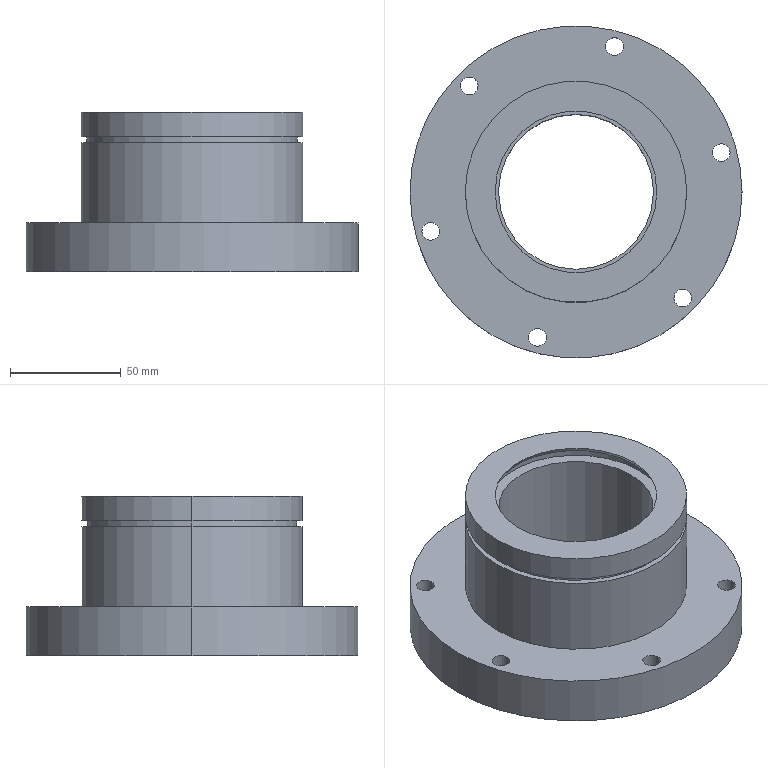Part | SolidWorks | features ICE 3, Chamfer 1, Extrusion 1, RevCut 1 | 1 solid | 45 faces | box 150 x 150 x 72 mm | volume 489629 mm3 | cylinder 24 | cone 14 | plane 7 | commonest cylinder face diameters 8 x12 100 x4 70 x2 80 x2 95 x2 150 x2
STEP:
#1=CARTESIAN_POINT('',(-40.,0.,65.7));
#2=VERTEX_POINT('',#1);
#3=CARTESIAN_POINT('',(40.,0.,65.7));
#4=VERTEX_POINT('',#3);
#5=CARTESIAN_POINT('',(0.,0.,65.7));
#6=DIRECTION('',(0.,0.,1.));
#7=DIRECTION('',(1.,0.,0.));
#8=AXIS2_PLACEMENT_3D('',#5,#6,#7);
#9=CIRCLE('',#8,40.);
#10=EDGE_CURVE('',#2,#4,#9,.T.);
#11=ORIENTED_EDGE('',*,*,#10,.F.);
#12=CARTESIAN_POINT('',(-40.,0.,70.));
#13=VERTEX_POINT('',#12);
#14=CARTESIAN_POINT('',(-40.,0.,72.));
#15=DIRECTION('',(0.,0.,1.));
#16=VECTOR('',#15,1000.);
#17=LINE('',#14,#16);
#18=EDGE_CURVE('',#2,#13,#17,.T.);
#19=ORIENTED_EDGE('',*,*,#18,.T.);
#20=CARTESIAN_POINT('',(40.,0.,70.));
#21=VERTEX_POINT('',#20);
#22=CARTESIAN_POINT('',(0.,0.,70.));
#23=DIRECTION('',(0.,0.,1.));
#24=DIRECTION('',(1.,0.,0.));
#25=AXIS2_PLACEMENT_3D('',#22,#23,#24);
#26=CIRCLE('',#25,40.);
#27=EDGE_CURVE('',#13,#21,#26,.T.);
#28=ORIENTED_EDGE('',*,*,#27,.T.);
#29=CARTESIAN_POINT('',(40.,0.,72.));
#30=DIRECTION('',(0.,0.,1.));
#31=VECTOR('',#30,1000.);
#32=LINE('',#29,#31);
#33=EDGE_CURVE('',#4,#21,#32,.T.);
#34=ORIENTED_EDGE('',*,*,#33,.F.);
#35=EDGE_LOOP('',(#11,#19,#28,#34));
#36=FACE_OUTER_BOUND('',#35,.T.);
#37=CARTESIAN_POINT('',(0.,0.,72.));
#38=DIRECTION('',(0.,0.,1.));
#39=DIRECTION('',(1.,0.,0.));
#40=AXIS2_PLACEMENT_3D('',#37,#38,#39);
#41=CYLINDRICAL_SURFACE('',#40,40.);
#42=ADVANCED_FACE('',(#36),#41,.F.);
#43=CARTESIAN_POINT('',(-36.5,0.,72.));
#44=VERTEX_POINT('',#43);
#45=CARTESIAN_POINT('',(36.5,0.,72.));
#46=VERTEX_POINT('',#45);
#47=CARTESIAN_POINT('',(0.,0.,72.));
#48=DIRECTION('',(0.,0.,1.));
#49=DIRECTION('',(1.,0.,0.));
#50=AXIS2_PLACEMENT_3D('',#47,#48,#49);
#51=CIRCLE('',#50,36.5);
#52=EDGE_CURVE('',#44,#46,#51,.T.);
#53=ORIENTED_EDGE('',*,*,#52,.T.);
#54=CARTESIAN_POINT('',(37.655,0.,70.));
#55=VERTEX_POINT('',#54);
#56=CARTESIAN_POINT('',(37.655,0.,70.));
#57=DIRECTION('',(0.5,0.,-0.866));
#58=VECTOR('',#57,1000.);
#59=LINE('',#56,#58);
#60=EDGE_CURVE('',#46,#55,#59,.T.);
#61=ORIENTED_EDGE('',*,*,#60,.T.);
#62=CARTESIAN_POINT('',(-37.655,0.,70.));
#63=VERTEX_POINT('',#62);
#64=CARTESIAN_POINT('',(0.,0.,70.));
#65=DIRECTION('',(0.,0.,1.));
#66=DIRECTION('',(1.,0.,0.));
#67=AXIS2_PLACEMENT_3D('',#64,#65,#66);
#68=CIRCLE('',#67,37.655);
#69=EDGE_CURVE('',#63,#55,#68,.T.);
#70=ORIENTED_EDGE('',*,*,#69,.F.);
#71=CARTESIAN_POINT('',(-37.655,0.,70.));
#72=DIRECTION('',(-0.5,0.,-0.866));
#73=VECTOR('',#72,1000.);
#74=LINE('',#71,#73);
#75=EDGE_CURVE('',#44,#63,#74,.T.);
#76=ORIENTED_EDGE('',*,*,#75,.F.);
#77=EDGE_LOOP('',(#53,#61,#70,#76));
#78=FACE_OUTER_BOUND('',#77,.T.);
#79=CARTESIAN_POINT('',(0.,0.,70.));
#80=DIRECTION('',(0.,0.,-1.));
#81=DIRECTION('',(-1.,0.,0.));
#82=AXIS2_PLACEMENT_3D('',#79,#80,#81);
#83=CONICAL_SURFACE('',#82,37.655,0.5236);
#84=ADVANCED_FACE('',(#78),#83,.F.);
#85=CARTESIAN_POINT('',(21.414,65.732,1.));
#86=VERTEX_POINT('',#85);
#87=CARTESIAN_POINT('',(13.414,65.732,1.));
#88=VERTEX_POINT('',#87);
#89=CARTESIAN_POINT('',(17.414,65.732,1.));
#90=DIRECTION('',(0.,0.,-1.));
#91=DIRECTION('',(1.,0.,0.));
#92=AXIS2_PLACEMENT_3D('',#89,#90,#91);
#93=CIRCLE('',#92,4.);
#94=EDGE_CURVE('',#86,#88,#93,.T.);
#95=ORIENTED_EDGE('',*,*,#94,.F.);
#96=CARTESIAN_POINT('',(22.414,65.732,0.));
#97=VERTEX_POINT('',#96);
#98=CARTESIAN_POINT('',(21.414,65.732,1.));
#99=DIRECTION('',(0.7071,0.,-0.7071));
#100=VECTOR('',#99,1000.);
#101=LINE('',#98,#100);
#102=EDGE_CURVE('',#86,#97,#101,.T.);
#103=ORIENTED_EDGE('',*,*,#102,.T.);
#104=CARTESIAN_POINT('',(12.414,65.732,0.));
#105=VERTEX_POINT('',#104);
#106=CARTESIAN_POINT('',(17.414,65.732,0.));
#107=DIRECTION('',(0.,0.,1.));
#108=DIRECTION('',(1.,0.,0.));
#109=AXIS2_PLACEMENT_3D('',#106,#107,#108);
#110=CIRCLE('',#109,5.);
#111=EDGE_CURVE('',#105,#97,#110,.T.);
#112=ORIENTED_EDGE('',*,*,#111,.F.);
#113=CARTESIAN_POINT('',(13.414,65.732,1.));
#114=DIRECTION('',(-0.7071,0.,-0.7071));
#115=VECTOR('',#114,1000.);
#116=LINE('',#113,#115);
#117=EDGE_CURVE('',#88,#105,#116,.T.);
#118=ORIENTED_EDGE('',*,*,#117,.F.);
#119=EDGE_LOOP('',(#95,#103,#112,#118));
#120=FACE_OUTER_BOUND('',#119,.T.);
#121=CARTESIAN_POINT('',(17.414,65.732,1.));
#122=DIRECTION('',(0.,0.,-1.));
#123=DIRECTION('',(-1.,0.,0.));
#124=AXIS2_PLACEMENT_3D('',#121,#122,#123);
#125=CONICAL_SURFACE('',#124,4.,0.7854);
#126=ADVANCED_FACE('',(#120),#125,.F.);
#127=CARTESIAN_POINT('',(69.633,17.785,1.));
#128=VERTEX_POINT('',#127);
#129=CARTESIAN_POINT('',(61.633,17.785,1.));
#130=VERTEX_POINT('',#129);
#131=CARTESIAN_POINT('',(65.633,17.785,1.));
#132=DIRECTION('',(0.,0.,-1.));
#133=DIRECTION('',(1.,0.,0.));
#134=AXIS2_PLACEMENT_3D('',#131,#132,#133);
#135=CIRCLE('',#134,4.);
#136=EDGE_CURVE('',#128,#130,#135,.T.);
#137=ORIENTED_EDGE('',*,*,#136,.F.);
#138=CARTESIAN_POINT('',(70.633,17.785,0.));
#139=VERTEX_POINT('',#138);
#140=CARTESIAN_POINT('',(69.633,17.785,1.));
#141=DIRECTION('',(0.7071,0.,-0.7071));
#142=VECTOR('',#141,1000.);
#143=LINE('',#140,#142);
#144=EDGE_CURVE('',#128,#139,#143,.T.);
#145=ORIENTED_EDGE('',*,*,#144,.T.);
#146=CARTESIAN_POINT('',(60.633,17.785,0.));
#147=VERTEX_POINT('',#146);
#148=CARTESIAN_POINT('',(65.633,17.785,0.));
#149=DIRECTION('',(0.,0.,1.));
#150=DIRECTION('',(1.,0.,0.));
#151=AXIS2_PLACEMENT_3D('',#148,#149,#150);
#152=CIRCLE('',#151,5.);
#153=EDGE_CURVE('',#147,#139,#152,.T.);
#154=ORIENTED_EDGE('',*,*,#153,.F.);
#155=CARTESIAN_POINT('',(61.633,17.785,1.));
#156=DIRECTION('',(-0.7071,0.,-0.7071));
#157=VECTOR('',#156,1000.);
#158=LINE('',#155,#157);
#159=EDGE_CURVE('',#130,#147,#158,.T.);
#160=ORIENTED_EDGE('',*,*,#159,.F.);
#161=EDGE_LOOP('',(#137,#145,#154,#160));
#162=FACE_OUTER_BOUND('',#161,.T.);
#163=CARTESIAN_POINT('',(65.633,17.785,1.));
#164=DIRECTION('',(0.,0.,-1.));
#165=DIRECTION('',(-1.,0.,0.));
#166=AXIS2_PLACEMENT_3D('',#163,#164,#165);
#167=CONICAL_SURFACE('',#166,4.,0.7854);
#168=ADVANCED_FACE('',(#162),#167,.F.);
#169=CARTESIAN_POINT('',(-44.219,47.947,1.));
#170=VERTEX_POINT('',#169);
#171=CARTESIAN_POINT('',(-52.219,47.947,1.));
#172=VERTEX_POINT('',#171);
#173=CARTESIAN_POINT('',(-48.219,47.947,1.));
#174=DIRECTION('',(0.,0.,-1.));
#175=DIRECTION('',(1.,0.,0.));
#176=AXIS2_PLACEMENT_3D('',#173,#174,#175);
#177=CIRCLE('',#176,4.);
#178=EDGE_CURVE('',#170,#172,#177,.T.);
#179=ORIENTED_EDGE('',*,*,#178,.F.);
#180=CARTESIAN_POINT('',(-43.219,47.947,0.));
#181=VERTEX_POINT('',#180);
#182=CARTESIAN_POINT('',(-44.219,47.947,1.));
#183=DIRECTION('',(0.7071,0.,-0.7071));
#184=VECTOR('',#183,1000.);
#185=LINE('',#182,#184);
#186=EDGE_CURVE('',#170,#181,#185,.T.);
#187=ORIENTED_EDGE('',*,*,#186,.T.);
#188=CARTESIAN_POINT('',(-53.219,47.947,0.));
#189=VERTEX_POINT('',#188);
#190=CARTESIAN_POINT('',(-48.219,47.947,0.));
#191=DIRECTION('',(0.,0.,1.));
#192=DIRECTION('',(1.,0.,0.));
#193=AXIS2_PLACEMENT_3D('',#190,#191,#192);
#194=CIRCLE('',#193,5.);
#195=EDGE_CURVE('',#189,#181,#194,.T.);
#196=ORIENTED_EDGE('',*,*,#195,.F.);
#197=CARTESIAN_POINT('',(-52.219,47.947,1.));
#198=DIRECTION('',(-0.7071,0.,-0.7071));
#199=VECTOR('',#198,1000.);
#200=LINE('',#197,#199);
#201=EDGE_CURVE('',#172,#189,#200,.T.);
#202=ORIENTED_EDGE('',*,*,#201,.F.);
#203=EDGE_LOOP('',(#179,#187,#196,#202));
#204=FACE_OUTER_BOUND('',#203,.T.);
#205=CARTESIAN_POINT('',(-48.219,47.947,1.));
#206=DIRECTION('',(0.,0.,-1.));
#207=DIRECTION('',(-1.,0.,0.));
#208=AXIS2_PLACEMENT_3D('',#205,#206,#207);
#209=CONICAL_SURFACE('',#208,4.,0.7854);
#210=ADVANCED_FACE('',(#204),#209,.F.);
#211=CARTESIAN_POINT('',(-61.633,-17.785,1.));
#212=VERTEX_POINT('',#211);
#213=CARTESIAN_POINT('',(-69.633,-17.785,1.));
#214=VERTEX_POINT('',#213);
#215=CARTESIAN_POINT('',(-65.633,-17.785,1.));
#216=DIRECTION('',(0.,0.,-1.));
#217=DIRECTION('',(1.,0.,0.));
#218=AXIS2_PLACEMENT_3D('',#215,#216,#217);
#219=CIRCLE('',#218,4.);
#220=EDGE_CURVE('',#212,#214,#219,.T.);
#221=ORIENTED_EDGE('',*,*,#220,.F.);
#222=CARTESIAN_POINT('',(-60.633,-17.785,0.));
#223=VERTEX_POINT('',#222);
#224=CARTESIAN_POINT('',(-61.633,-17.785,1.));
#225=DIRECTION('',(0.7071,0.,-0.7071));
#226=VECTOR('',#225,1000.);
#227=LINE('',#224,#226);
#228=EDGE_CURVE('',#212,#223,#227,.T.);
#229=ORIENTED_EDGE('',*,*,#228,.T.);
#230=CARTESIAN_POINT('',(-70.633,-17.785,0.));
#231=VERTEX_POINT('',#230);
#232=CARTESIAN_POINT('',(-65.633,-17.785,0.));
#233=DIRECTION('',(0.,0.,1.));
#234=DIRECTION('',(1.,0.,0.));
#235=AXIS2_PLACEMENT_3D('',#232,#233,#234);
#236=CIRCLE('',#235,5.);
#237=EDGE_CURVE('',#231,#223,#236,.T.);
#238=ORIENTED_EDGE('',*,*,#237,.F.);
#239=CARTESIAN_POINT('',(-69.633,-17.785,1.));
#240=DIRECTION('',(-0.7071,0.,-0.7071));
#241=VECTOR('',#240,1000.);
#242=LINE('',#239,#241);
#243=EDGE_CURVE('',#214,#231,#242,.T.);
#244=ORIENTED_EDGE('',*,*,#243,.F.);
#245=EDGE_LOOP('',(#221,#229,#238,#244));
#246=FACE_OUTER_BOUND('',#245,.T.);
#247=CARTESIAN_POINT('',(-65.633,-17.785,1.));
#248=DIRECTION('',(0.,0.,-1.));
#249=DIRECTION('',(-1.,0.,0.));
#250=AXIS2_PLACEMENT_3D('',#247,#248,#249);
#251=CONICAL_SURFACE('',#250,4.,0.7854);
#252=ADVANCED_FACE('',(#246),#251,.F.);
#253=CARTESIAN_POINT('',(-13.414,-65.732,1.));
#254=VERTEX_POINT('',#253);
#255=CARTESIAN_POINT('',(-21.414,-65.732,1.));
#256=VERTEX_POINT('',#255);
#257=CARTESIAN_POINT('',(-17.414,-65.732,1.));
#258=DIRECTION('',(0.,0.,-1.));
#259=DIRECTION('',(1.,0.,0.));
#260=AXIS2_PLACEMENT_3D('',#257,#258,#259);
#261=CIRCLE('',#260,4.);
#262=EDGE_CURVE('',#254,#256,#261,.T.);
#263=ORIENTED_EDGE('',*,*,#262,.F.);
#264=CARTESIAN_POINT('',(-12.414,-65.732,0.));
#265=VERTEX_POINT('',#264);
#266=CARTESIAN_POINT('',(-13.414,-65.732,1.));
#267=DIRECTION('',(0.7071,0.,-0.7071));
#268=VECTOR('',#267,1000.);
#269=LINE('',#266,#268);
#270=EDGE_CURVE('',#254,#265,#269,.T.);
#271=ORIENTED_EDGE('',*,*,#270,.T.);
#272=CARTESIAN_POINT('',(-22.414,-65.732,0.));
#273=VERTEX_POINT('',#272);
#274=CARTESIAN_POINT('',(-17.414,-65.732,0.));
#275=DIRECTION('',(0.,0.,1.));
#276=DIRECTION('',(1.,0.,0.));
#277=AXIS2_PLACEMENT_3D('',#274,#275,#276);
#278=CIRCLE('',#277,5.);
#279=EDGE_CURVE('',#273,#265,#278,.T.);
#280=ORIENTED_EDGE('',*,*,#279,.F.);
#281=CARTESIAN_POINT('',(-21.414,-65.732,1.));
#282=DIRECTION('',(-0.7071,0.,-0.7071));
#283=VECTOR('',#282,1000.);
#284=LINE('',#281,#283);
#285=EDGE_CURVE('',#256,#273,#284,.T.);
#286=ORIENTED_EDGE('',*,*,#285,.F.);
#287=EDGE_LOOP('',(#263,#271,#280,#286));
#288=FACE_OUTER_BOUND('',#287,.T.);
#289=CARTESIAN_POINT('',(-17.414,-65.732,1.));
#290=DIRECTION('',(0.,0.,-1.));
#291=DIRECTION('',(-1.,0.,0.));
#292=AXIS2_PLACEMENT_3D('',#289,#290,#291);
#293=CONICAL_SURFACE('',#292,4.,0.7854);
#294=ADVANCED_FACE('',(#288),#293,.F.);
#295=CARTESIAN_POINT('',(52.219,-47.947,1.));
#296=VERTEX_POINT('',#295);
#297=CARTESIAN_POINT('',(44.219,-47.947,1.));
#298=VERTEX_POINT('',#297);
#299=CARTESIAN_POINT('',(48.219,-47.947,1.));
#300=DIRECTION('',(0.,0.,-1.));
#301=DIRECTION('',(1.,0.,0.));
#302=AXIS2_PLACEMENT_3D('',#299,#300,#301);
#303=CIRCLE('',#302,4.);
#304=EDGE_CURVE('',#296,#298,#303,.T.);
#305=ORIENTED_EDGE('',*,*,#304,.F.);
#306=CARTESIAN_POINT('',(53.219,-47.947,0.));
#307=VERTEX_POINT('',#306);
#308=CARTESIAN_POINT('',(52.219,-47.947,1.));
#309=DIRECTION('',(0.7071,0.,-0.7071));
#310=VECTOR('',#309,1000.);
#311=LINE('',#308,#310);
#312=EDGE_CURVE('',#296,#307,#311,.T.);
#313=ORIENTED_EDGE('',*,*,#312,.T.);
#314=CARTESIAN_POINT('',(43.219,-47.947,0.));
#315=VERTEX_POINT('',#314);
#316=CARTESIAN_POINT('',(48.219,-47.947,0.));
#317=DIRECTION('',(0.,0.,1.));
#318=DIRECTION('',(1.,0.,0.));
#319=AXIS2_PLACEMENT_3D('',#316,#317,#318);
#320=CIRCLE('',#319,5.);
#321=EDGE_CURVE('',#315,#307,#320,.T.);
#322=ORIENTED_EDGE('',*,*,#321,.F.);
#323=CARTESIAN_POINT('',(44.219,-47.947,1.));
#324=DIRECTION('',(-0.7071,0.,-0.7071));
#325=VECTOR('',#324,1000.);
#326=LINE('',#323,#325);
#327=EDGE_CURVE('',#298,#315,#326,.T.);
#328=ORIENTED_EDGE('',*,*,#327,.F.);
#329=EDGE_LOOP('',(#305,#313,#322,#328));
#330=FACE_OUTER_BOUND('',#329,.T.);
#331=CARTESIAN_POINT('',(48.219,-47.947,1.));
#332=DIRECTION('',(0.,0.,-1.));
#333=DIRECTION('',(-1.,0.,0.));
#334=AXIS2_PLACEMENT_3D('',#331,#332,#333);
#335=CONICAL_SURFACE('',#334,4.,0.7854);
#336=ADVANCED_FACE('',(#330),#335,.F.);
#337=CARTESIAN_POINT('',(13.414,65.732,22.));
#338=VERTEX_POINT('',#337);
#339=CARTESIAN_POINT('',(21.414,65.732,22.));
#340=VERTEX_POINT('',#339);
#341=CARTESIAN_POINT('',(17.414,65.732,22.));
#342=DIRECTION('',(0.,0.,1.));
#343=DIRECTION('',(1.,0.,0.));
#344=AXIS2_PLACEMENT_3D('',#341,#342,#343);
#345=CIRCLE('',#344,4.);
#346=EDGE_CURVE('',#338,#340,#345,.T.);
#347=ORIENTED_EDGE('',*,*,#346,.T.);
#348=CARTESIAN_POINT('',(21.414,65.732,72.));
#349=DIRECTION('',(0.,0.,-1.));
#350=VECTOR('',#349,1000.);
#351=LINE('',#348,#350);
#352=EDGE_CURVE('',#340,#86,#351,.T.);
#353=ORIENTED_EDGE('',*,*,#352,.T.);
#354=ORIENTED_EDGE('',*,*,#94,.T.);
#355=CARTESIAN_POINT('',(13.414,65.732,72.));
#356=DIRECTION('',(0.,0.,-1.));
#357=VECTOR('',#356,1000.);
#358=LINE('',#355,#357);
#359=EDGE_CURVE('',#338,#88,#358,.T.);
#360=ORIENTED_EDGE('',*,*,#359,.F.);
#361=EDGE_LOOP('',(#347,#353,#354,#360));
#362=FACE_OUTER_BOUND('',#361,.T.);
#363=CARTESIAN_POINT('',(17.414,65.732,72.));
#364=DIRECTION('',(0.,0.,-1.));
#365=DIRECTION('',(-1.,0.,0.));
#366=AXIS2_PLACEMENT_3D('',#363,#364,#365);
#367=CYLINDRICAL_SURFACE('',#366,4.);
#368=ADVANCED_FACE('',(#362),#367,.F.);
#369=CARTESIAN_POINT('',(-52.219,47.947,22.));
#370=VERTEX_POINT('',#369);
#371=CARTESIAN_POINT('',(-44.219,47.947,22.));
#372=VERTEX_POINT('',#371);
#373=CARTESIAN_POINT('',(-48.219,47.947,22.));
#374=DIRECTION('',(0.,0.,1.));
#375=DIRECTION('',(1.,0.,0.));
#376=AXIS2_PLACEMENT_3D('',#373,#374,#375);
#377=CIRCLE('',#376,4.);
#378=EDGE_CURVE('',#370,#372,#377,.T.);
#379=ORIENTED_EDGE('',*,*,#378,.T.);
#380=CARTESIAN_POINT('',(-44.219,47.947,72.));
#381=DIRECTION('',(0.,0.,-1.));
#382=VECTOR('',#381,1000.);
#383=LINE('',#380,#382);
#384=EDGE_CURVE('',#372,#170,#383,.T.);
#385=ORIENTED_EDGE('',*,*,#384,.T.);
#386=ORIENTED_EDGE('',*,*,#178,.T.);
#387=CARTESIAN_POINT('',(-52.219,47.947,72.));
#388=DIRECTION('',(0.,0.,-1.));
#389=VECTOR('',#388,1000.);
#390=LINE('',#387,#389);
#391=EDGE_CURVE('',#370,#172,#390,.T.);
#392=ORIENTED_EDGE('',*,*,#391,.F.);
#393=EDGE_LOOP('',(#379,#385,#386,#392));
#394=FACE_OUTER_BOUND('',#393,.T.);
#395=CARTESIAN_POINT('',(-48.219,47.947,72.));
#396=DIRECTION('',(0.,0.,-1.));
#397=DIRECTION('',(-1.,0.,0.));
#398=AXIS2_PLACEMENT_3D('',#395,#396,#397);
#399=CYLINDRICAL_SURFACE('',#398,4.);
#400=ADVANCED_FACE('',(#394),#399,.F.);
#401=CARTESIAN_POINT('',(-69.633,-17.785,22.));
#402=VERTEX_POINT('',#401);
#403=CARTESIAN_POINT('',(-61.633,-17.785,22.));
#404=VERTEX_POINT('',#403);
#405=CARTESIAN_POINT('',(-65.633,-17.785,22.));
#406=DIRECTION('',(0.,0.,1.));
#407=DIRECTION('',(1.,0.,0.));
#408=AXIS2_PLACEMENT_3D('',#405,#406,#407);
#409=CIRCLE('',#408,4.);
#410=EDGE_CURVE('',#402,#404,#409,.T.);
#411=ORIENTED_EDGE('',*,*,#410,.T.);
#412=CARTESIAN_POINT('',(-61.633,-17.785,72.));
#413=DIRECTION('',(0.,0.,-1.));
#414=VECTOR('',#413,1000.);
#415=LINE('',#412,#414);
#416=EDGE_CURVE('',#404,#212,#415,.T.);
#417=ORIENTED_EDGE('',*,*,#416,.T.);
#418=ORIENTED_EDGE('',*,*,#220,.T.);
#419=CARTESIAN_POINT('',(-69.633,-17.785,72.));
#420=DIRECTION('',(0.,0.,-1.));
#421=VECTOR('',#420,1000.);
#422=LINE('',#419,#421);
#423=EDGE_CURVE('',#402,#214,#422,.T.);
#424=ORIENTED_EDGE('',*,*,#423,.F.);
#425=EDGE_LOOP('',(#411,#417,#418,#424));
#426=FACE_OUTER_BOUND('',#425,.T.);
#427=CARTESIAN_POINT('',(-65.633,-17.785,72.));
#428=DIRECTION('',(0.,0.,-1.));
#429=DIRECTION('',(-1.,0.,0.));
#430=AXIS2_PLACEMENT_3D('',#427,#428,#429);
#431=CYLINDRICAL_SURFACE('',#430,4.);
#432=ADVANCED_FACE('',(#426),#431,.F.);
#433=CARTESIAN_POINT('',(-21.414,-65.732,22.));
#434=VERTEX_POINT('',#433);
#435=CARTESIAN_POINT('',(-13.414,-65.732,22.));
#436=VERTEX_POINT('',#435);
#437=CARTESIAN_POINT('',(-17.414,-65.732,22.));
#438=DIRECTION('',(0.,0.,1.));
#439=DIRECTION('',(1.,0.,0.));
#440=AXIS2_PLACEMENT_3D('',#437,#438,#439);
#441=CIRCLE('',#440,4.);
#442=EDGE_CURVE('',#434,#436,#441,.T.);
#443=ORIENTED_EDGE('',*,*,#442,.T.);
#444=CARTESIAN_POINT('',(-13.414,-65.732,72.));
#445=DIRECTION('',(0.,0.,-1.));
#446=VECTOR('',#445,1000.);
#447=LINE('',#444,#446);
#448=EDGE_CURVE('',#436,#254,#447,.T.);
#449=ORIENTED_EDGE('',*,*,#448,.T.);
#450=ORIENTED_EDGE('',*,*,#262,.T.);
#451=CARTESIAN_POINT('',(-21.414,-65.732,72.));
#452=DIRECTION('',(0.,0.,-1.));
#453=VECTOR('',#452,1000.);
#454=LINE('',#451,#453);
#455=EDGE_CURVE('',#434,#256,#454,.T.);
#456=ORIENTED_EDGE('',*,*,#455,.F.);
#457=EDGE_LOOP('',(#443,#449,#450,#456));
#458=FACE_OUTER_BOUND('',#457,.T.);
#459=CARTESIAN_POINT('',(-17.414,-65.732,72.));
#460=DIRECTION('',(0.,0.,-1.));
#461=DIRECTION('',(-1.,0.,0.));
#462=AXIS2_PLACEMENT_3D('',#459,#460,#461);
#463=CYLINDRICAL_SURFACE('',#462,4.);
#464=ADVANCED_FACE('',(#458),#463,.F.);
#465=CARTESIAN_POINT('',(44.219,-47.947,22.));
#466=VERTEX_POINT('',#465);
#467=CARTESIAN_POINT('',(52.219,-47.947,22.));
#468=VERTEX_POINT('',#467);
#469=CARTESIAN_POINT('',(48.219,-47.947,22.));
#470=DIRECTION('',(0.,0.,1.));
#471=DIRECTION('',(1.,0.,0.));
#472=AXIS2_PLACEMENT_3D('',#469,#470,#471);
#473=CIRCLE('',#472,4.);
#474=EDGE_CURVE('',#466,#468,#473,.T.);
#475=ORIENTED_EDGE('',*,*,#474,.T.);
#476=CARTESIAN_POINT('',(52.219,-47.947,72.));
#477=DIRECTION('',(0.,0.,-1.));
#478=VECTOR('',#477,1000.);
#479=LINE('',#476,#478);
#480=EDGE_CURVE('',#468,#296,#479,.T.);
#481=ORIENTED_EDGE('',*,*,#480,.T.);
#482=ORIENTED_EDGE('',*,*,#304,.T.);
#483=CARTESIAN_POINT('',(44.219,-47.947,72.));
#484=DIRECTION('',(0.,0.,-1.));
#485=VECTOR('',#484,1000.);
#486=LINE('',#483,#485);
#487=EDGE_CURVE('',#466,#298,#486,.T.);
#488=ORIENTED_EDGE('',*,*,#487,.F.);
#489=EDGE_LOOP('',(#475,#481,#482,#488));
#490=FACE_OUTER_BOUND('',#489,.T.);
#491=CARTESIAN_POINT('',(48.219,-47.947,72.));
#492=DIRECTION('',(0.,0.,-1.));
#493=DIRECTION('',(-1.,0.,0.));
#494=AXIS2_PLACEMENT_3D('',#491,#492,#493);
#495=CYLINDRICAL_SURFACE('',#494,4.);
#496=ADVANCED_FACE('',(#490),#495,.F.);
#497=CARTESIAN_POINT('',(61.633,17.785,22.));
#498=VERTEX_POINT('',#497);
#499=CARTESIAN_POINT('',(69.633,17.785,22.));
#500=VERTEX_POINT('',#499);
#501=CARTESIAN_POINT('',(65.633,17.785,22.));
#502=DIRECTION('',(0.,0.,1.));
#503=DIRECTION('',(1.,0.,0.));
#504=AXIS2_PLACEMENT_3D('',#501,#502,#503);
#505=CIRCLE('',#504,4.);
#506=EDGE_CURVE('',#498,#500,#505,.T.);
#507=ORIENTED_EDGE('',*,*,#506,.T.);
#508=CARTESIAN_POINT('',(69.633,17.785,72.));
#509=DIRECTION('',(0.,0.,-1.));
#510=VECTOR('',#509,1000.);
#511=LINE('',#508,#510);
#512=EDGE_CURVE('',#500,#128,#511,.T.);
#513=ORIENTED_EDGE('',*,*,#512,.T.);
#514=ORIENTED_EDGE('',*,*,#136,.T.);
#515=CARTESIAN_POINT('',(61.633,17.785,72.));
#516=DIRECTION('',(0.,0.,-1.));
#517=VECTOR('',#516,1000.);
#518=LINE('',#515,#517);
#519=EDGE_CURVE('',#498,#130,#518,.T.);
#520=ORIENTED_EDGE('',*,*,#519,.F.);
#521=EDGE_LOOP('',(#507,#513,#514,#520));
#522=FACE_OUTER_BOUND('',#521,.T.);
#523=CARTESIAN_POINT('',(65.633,17.785,72.));
#524=DIRECTION('',(0.,0.,-1.));
#525=DIRECTION('',(-1.,0.,0.));
#526=AXIS2_PLACEMENT_3D('',#523,#524,#525);
#527=CYLINDRICAL_SURFACE('',#526,4.);
#528=ADVANCED_FACE('',(#522),#527,.F.);
#529=CARTESIAN_POINT('',(47.5,0.,58.35));
#530=VERTEX_POINT('',#529);
#531=CARTESIAN_POINT('',(-47.5,0.,58.35));
#532=VERTEX_POINT('',#531);
#533=CARTESIAN_POINT('',(0.,0.,58.35));
#534=DIRECTION('',(0.,0.,1.));
#535=DIRECTION('',(1.,0.,0.));
#536=AXIS2_PLACEMENT_3D('',#533,#534,#535);
#537=CIRCLE('',#536,47.5);
#538=EDGE_CURVE('',#530,#532,#537,.T.);
#539=ORIENTED_EDGE('',*,*,#538,.T.);
#540=CARTESIAN_POINT('',(-47.5,0.,61.));
#541=VERTEX_POINT('',#540);
#542=CARTESIAN_POINT('',(-47.5,0.,58.35));
#543=DIRECTION('',(0.,0.,1.));
#544=VECTOR('',#543,1000.);
#545=LINE('',#542,#544);
#546=EDGE_CURVE('',#532,#541,#545,.T.);
#547=ORIENTED_EDGE('',*,*,#546,.T.);
#548=CARTESIAN_POINT('',(47.5,0.,61.));
#549=VERTEX_POINT('',#548);
#550=CARTESIAN_POINT('',(0.,0.,61.));
#551=DIRECTION('',(0.,0.,1.));
#552=DIRECTION('',(1.,0.,0.));
#553=AXIS2_PLACEMENT_3D('',#550,#551,#552);
#554=CIRCLE('',#553,47.5);
#555=EDGE_CURVE('',#549,#541,#554,.T.);
#556=ORIENTED_EDGE('',*,*,#555,.F.);
#557=CARTESIAN_POINT('',(47.5,0.,58.35));
#558=DIRECTION('',(0.,0.,1.));
#559=VECTOR('',#558,1000.);
#560=LINE('',#557,#559);
#561=EDGE_CURVE('',#530,#549,#560,.T.);
#562=ORIENTED_EDGE('',*,*,#561,.F.);
#563=EDGE_LOOP('',(#539,#547,#556,#562));
#564=FACE_OUTER_BOUND('',#563,.T.);
#565=CARTESIAN_POINT('',(0.,0.,58.35));
#566=DIRECTION('',(0.,0.,1.));
#567=DIRECTION('',(1.,0.,0.));
#568=AXIS2_PLACEMENT_3D('',#565,#566,#567);
#569=CYLINDRICAL_SURFACE('',#568,47.5);
#570=ADVANCED_FACE('',(#564),#569,.T.);
#571=CARTESIAN_POINT('',(50.,0.,72.));
#572=VERTEX_POINT('',#571);
#573=CARTESIAN_POINT('',(-50.,0.,72.));
#574=VERTEX_POINT('',#573);
#575=CARTESIAN_POINT('',(0.,0.,72.));
#576=DIRECTION('',(0.,0.,1.));
#577=DIRECTION('',(1.,0.,0.));
#578=AXIS2_PLACEMENT_3D('',#575,#576,#577);
#579=CIRCLE('',#578,50.);
#580=EDGE_CURVE('',#572,#574,#579,.T.);
#581=ORIENTED_EDGE('',*,*,#580,.F.);
#582=CARTESIAN_POINT('',(50.,0.,61.));
#583=VERTEX_POINT('',#582);
#584=CARTESIAN_POINT('',(50.,0.,72.));
#585=DIRECTION('',(0.,0.,-1.));
#586=VECTOR('',#585,1000.);
#587=LINE('',#584,#586);
#588=EDGE_CURVE('',#572,#583,#587,.T.);
#589=ORIENTED_EDGE('',*,*,#588,.T.);
#590=CARTESIAN_POINT('',(-50.,0.,61.));
#591=VERTEX_POINT('',#590);
#592=CARTESIAN_POINT('',(0.,0.,61.));
#593=DIRECTION('',(0.,0.,1.));
#594=DIRECTION('',(1.,0.,0.));
#595=AXIS2_PLACEMENT_3D('',#592,#593,#594);
#596=CIRCLE('',#595,50.);
#597=EDGE_CURVE('',#583,#591,#596,.T.);
#598=ORIENTED_EDGE('',*,*,#597,.T.);
#599=CARTESIAN_POINT('',(-50.,0.,72.));
#600=DIRECTION('',(0.,0.,-1.));
#601=VECTOR('',#600,1000.);
#602=LINE('',#599,#601);
#603=EDGE_CURVE('',#574,#591,#602,.T.);
#604=ORIENTED_EDGE('',*,*,#603,.F.);
#605=EDGE_LOOP('',(#581,#589,#598,#604));
#606=FACE_OUTER_BOUND('',#605,.T.);
#607=CARTESIAN_POINT('',(0.,0.,72.));
#608=DIRECTION('',(0.,0.,-1.));
#609=DIRECTION('',(-1.,0.,0.));
#610=AXIS2_PLACEMENT_3D('',#607,#608,#609);
#611=CYLINDRICAL_SURFACE('',#610,50.);
#612=ADVANCED_FACE('',(#606),#611,.T.);
#613=CARTESIAN_POINT('',(75.,0.,22.));
#614=VERTEX_POINT('',#613);
#615=CARTESIAN_POINT('',(-75.,0.,22.));
#616=VERTEX_POINT('',#615);
#617=CARTESIAN_POINT('',(0.,0.,22.));
#618=DIRECTION('',(0.,0.,1.));
#619=DIRECTION('',(1.,0.,0.));
#620=AXIS2_PLACEMENT_3D('',#617,#618,#619);
#621=CIRCLE('',#620,75.);
#622=EDGE_CURVE('',#614,#616,#621,.T.);
#623=ORIENTED_EDGE('',*,*,#622,.F.);
#624=CARTESIAN_POINT('',(75.,0.,0.));
#625=VERTEX_POINT('',#624);
#626=CARTESIAN_POINT('',(75.,0.,22.));
#627=DIRECTION('',(0.,0.,-1.));
#628=VECTOR('',#627,1000.);
#629=LINE('',#626,#628);
#630=EDGE_CURVE('',#614,#625,#629,.T.);
#631=ORIENTED_EDGE('',*,*,#630,.T.);
#632=CARTESIAN_POINT('',(-75.,0.,0.));
#633=VERTEX_POINT('',#632);
#634=CARTESIAN_POINT('',(0.,0.,0.));
#635=DIRECTION('',(0.,0.,1.));
#636=DIRECTION('',(1.,0.,0.));
#637=AXIS2_PLACEMENT_3D('',#634,#635,#636);
#638=CIRCLE('',#637,75.);
#639=EDGE_CURVE('',#625,#633,#638,.T.);
#640=ORIENTED_EDGE('',*,*,#639,.T.);
#641=CARTESIAN_POINT('',(-75.,0.,22.));
#642=DIRECTION('',(0.,0.,-1.));
#643=VECTOR('',#642,1000.);
#644=LINE('',#641,#643);
#645=EDGE_CURVE('',#616,#633,#644,.T.);
#646=ORIENTED_EDGE('',*,*,#645,.F.);
#647=EDGE_LOOP('',(#623,#631,#640,#646));
#648=FACE_OUTER_BOUND('',#647,.T.);
#649=CARTESIAN_POINT('',(0.,0.,22.));
#650=DIRECTION('',(0.,0.,-1.));
#651=DIRECTION('',(-1.,0.,0.));
#652=AXIS2_PLACEMENT_3D('',#649,#650,#651);
#653=CYLINDRICAL_SURFACE('',#652,75.);
#654=ADVANCED_FACE('',(#648),#653,.T.);
#655=CARTESIAN_POINT('',(50.,0.,58.35));
#656=VERTEX_POINT('',#655);
#657=CARTESIAN_POINT('',(-50.,0.,58.35));
#658=VERTEX_POINT('',#657);
#659=CARTESIAN_POINT('',(0.,0.,58.35));
#660=DIRECTION('',(0.,0.,1.));
#661=DIRECTION('',(1.,0.,0.));
#662=AXIS2_PLACEMENT_3D('',#659,#660,#661);
#663=CIRCLE('',#662,50.);
#664=EDGE_CURVE('',#656,#658,#663,.T.);
#665=ORIENTED_EDGE('',*,*,#664,.F.);
#666=CARTESIAN_POINT('',(50.,0.,22.));
#667=VERTEX_POINT('',#666);
#668=CARTESIAN_POINT('',(50.,0.,72.));
#669=DIRECTION('',(0.,0.,-1.));
#670=VECTOR('',#669,1000.);
#671=LINE('',#668,#670);
#672=EDGE_CURVE('',#656,#667,#671,.T.);
#673=ORIENTED_EDGE('',*,*,#672,.T.);
#674=CARTESIAN_POINT('',(-50.,0.,22.));
#675=VERTEX_POINT('',#674);
#676=CARTESIAN_POINT('',(0.,0.,22.));
#677=DIRECTION('',(0.,0.,1.));
#678=DIRECTION('',(1.,0.,0.));
#679=AXIS2_PLACEMENT_3D('',#676,#677,#678);
#680=CIRCLE('',#679,50.);
#681=EDGE_CURVE('',#667,#675,#680,.T.);
#682=ORIENTED_EDGE('',*,*,#681,.T.);
#683=CARTESIAN_POINT('',(-50.,0.,72.));
#684=DIRECTION('',(0.,0.,-1.));
#685=VECTOR('',#684,1000.);
#686=LINE('',#683,#685);
#687=EDGE_CURVE('',#658,#675,#686,.T.);
#688=ORIENTED_EDGE('',*,*,#687,.F.);
#689=EDGE_LOOP('',(#665,#673,#682,#688));
#690=FACE_OUTER_BOUND('',#689,.T.);
#691=CARTESIAN_POINT('',(0.,0.,72.));
#692=DIRECTION('',(0.,0.,-1.));
#693=DIRECTION('',(-1.,0.,0.));
#694=AXIS2_PLACEMENT_3D('',#691,#692,#693);
#695=CYLINDRICAL_SURFACE('',#694,50.);
#696=ADVANCED_FACE('',(#690),#695,.T.);
#697=CARTESIAN_POINT('',(-35.,0.,65.7));
#698=VERTEX_POINT('',#697);
#699=CARTESIAN_POINT('',(35.,0.,65.7));
#700=VERTEX_POINT('',#699);
#701=CARTESIAN_POINT('',(0.,0.,65.7));
#702=DIRECTION('',(0.,0.,1.));
#703=DIRECTION('',(1.,0.,0.));
#704=AXIS2_PLACEMENT_3D('',#701,#702,#703);
#705=CIRCLE('',#704,35.);
#706=EDGE_CURVE('',#698,#700,#705,.T.);
#707=ORIENTED_EDGE('',*,*,#706,.T.);
#708=CARTESIAN_POINT('',(35.,0.,0.));
#709=VERTEX_POINT('',#708);
#710=CARTESIAN_POINT('',(35.,0.,22.));
#711=DIRECTION('',(0.,0.,-1.));
#712=VECTOR('',#711,1000.);
#713=LINE('',#710,#712);
#714=EDGE_CURVE('',#700,#709,#713,.T.);
#715=ORIENTED_EDGE('',*,*,#714,.T.);
#716=CARTESIAN_POINT('',(-35.,0.,0.));
#717=VERTEX_POINT('',#716);
#718=CARTESIAN_POINT('',(0.,0.,0.));
#719=DIRECTION('',(0.,0.,1.));
#720=DIRECTION('',(1.,0.,0.));
#721=AXIS2_PLACEMENT_3D('',#718,#719,#720);
#722=CIRCLE('',#721,35.);
#723=EDGE_CURVE('',#717,#709,#722,.T.);
#724=ORIENTED_EDGE('',*,*,#723,.F.);
#725=CARTESIAN_POINT('',(-35.,0.,22.));
#726=DIRECTION('',(0.,0.,-1.));
#727=VECTOR('',#726,1000.);
#728=LINE('',#725,#727);
#729=EDGE_CURVE('',#698,#717,#728,.T.);
#730=ORIENTED_EDGE('',*,*,#729,.F.);
#731=EDGE_LOOP('',(#707,#715,#724,#730));
#732=FACE_OUTER_BOUND('',#731,.T.);
#733=CARTESIAN_POINT('',(0.,0.,22.));
#734=DIRECTION('',(0.,0.,-1.));
#735=DIRECTION('',(-1.,0.,0.));
#736=AXIS2_PLACEMENT_3D('',#733,#734,#735);
#737=CYLINDRICAL_SURFACE('',#736,35.);
#738=ADVANCED_FACE('',(#732),#737,.F.);
#739=ORIENTED_EDGE('',*,*,#714,.F.);
#740=CARTESIAN_POINT('',(0.,0.,65.7));
#741=DIRECTION('',(0.,0.,1.));
#742=DIRECTION('',(1.,0.,0.));
#743=AXIS2_PLACEMENT_3D('',#740,#741,#742);
#744=CIRCLE('',#743,35.);
#745=EDGE_CURVE('',#700,#698,#744,.T.);
#746=ORIENTED_EDGE('',*,*,#745,.T.);
#747=ORIENTED_EDGE('',*,*,#729,.T.);
#748=CARTESIAN_POINT('',(0.,0.,0.));
#749=DIRECTION('',(0.,0.,1.));
#750=DIRECTION('',(1.,0.,0.));
#751=AXIS2_PLACEMENT_3D('',#748,#749,#750);
#752=CIRCLE('',#751,35.);
#753=EDGE_CURVE('',#709,#717,#752,.T.);
#754=ORIENTED_EDGE('',*,*,#753,.F.);
#755=EDGE_LOOP('',(#739,#746,#747,#754));
#756=FACE_OUTER_BOUND('',#755,.T.);
#757=CARTESIAN_POINT('',(0.,0.,22.));
#758=DIRECTION('',(0.,0.,-1.));
#759=DIRECTION('',(-1.,0.,0.));
#760=AXIS2_PLACEMENT_3D('',#757,#758,#759);
#761=CYLINDRICAL_SURFACE('',#760,35.);
#762=ADVANCED_FACE('',(#756),#761,.F.);
#763=ORIENTED_EDGE('',*,*,#672,.F.);
#764=CARTESIAN_POINT('',(0.,0.,58.35));
#765=DIRECTION('',(0.,0.,1.));
#766=DIRECTION('',(1.,0.,0.));
#767=AXIS2_PLACEMENT_3D('',#764,#765,#766);
#768=CIRCLE('',#767,50.);
#769=EDGE_CURVE('',#658,#656,#768,.T.);
#770=ORIENTED_EDGE('',*,*,#769,.F.);
#771=ORIENTED_EDGE('',*,*,#687,.T.);
#772=CARTESIAN_POINT('',(0.,0.,22.));
#773=DIRECTION('',(0.,0.,1.));
#774=DIRECTION('',(1.,0.,0.));
#775=AXIS2_PLACEMENT_3D('',#772,#773,#774);
#776=CIRCLE('',#775,50.);
#777=EDGE_CURVE('',#675,#667,#776,.T.);
#778=ORIENTED_EDGE('',*,*,#777,.T.);
#779=EDGE_LOOP('',(#763,#770,#771,#778));
#780=FACE_OUTER_BOUND('',#779,.T.);
#781=CARTESIAN_POINT('',(0.,0.,72.));
#782=DIRECTION('',(0.,0.,-1.));
#783=DIRECTION('',(-1.,0.,0.));
#784=AXIS2_PLACEMENT_3D('',#781,#782,#783);
#785=CYLINDRICAL_SURFACE('',#784,50.);
#786=ADVANCED_FACE('',(#780),#785,.T.);
#787=ORIENTED_EDGE('',*,*,#346,.F.);
#788=CARTESIAN_POINT('',(17.414,65.732,22.));
#789=DIRECTION('',(0.,0.,1.));
#790=DIRECTION('',(1.,0.,0.));
#791=AXIS2_PLACEMENT_3D('',#788,#789,#790);
#792=CIRCLE('',#791,4.);
#793=EDGE_CURVE('',#340,#338,#792,.T.);
#794=ORIENTED_EDGE('',*,*,#793,.F.);
#795=EDGE_LOOP('',(#787,#794));
#796=FACE_BOUND('',#795,.T.);
#797=ORIENTED_EDGE('',*,*,#378,.F.);
#798=CARTESIAN_POINT('',(-48.219,47.947,22.));
#799=DIRECTION('',(0.,0.,1.));
#800=DIRECTION('',(1.,0.,0.));
#801=AXIS2_PLACEMENT_3D('',#798,#799,#800);
#802=CIRCLE('',#801,4.);
#803=EDGE_CURVE('',#372,#370,#802,.T.);
#804=ORIENTED_EDGE('',*,*,#803,.F.);
#805=EDGE_LOOP('',(#797,#804));
#806=FACE_BOUND('',#805,.T.);
#807=ORIENTED_EDGE('',*,*,#410,.F.);
#808=CARTESIAN_POINT('',(-65.633,-17.785,22.));
#809=DIRECTION('',(0.,0.,1.));
#810=DIRECTION('',(1.,0.,0.));
#811=AXIS2_PLACEMENT_3D('',#808,#809,#810);
#812=CIRCLE('',#811,4.);
#813=EDGE_CURVE('',#404,#402,#812,.T.);
#814=ORIENTED_EDGE('',*,*,#813,.F.);
#815=EDGE_LOOP('',(#807,#814));
#816=FACE_BOUND('',#815,.T.);
#817=ORIENTED_EDGE('',*,*,#442,.F.);
#818=CARTESIAN_POINT('',(-17.414,-65.732,22.));
#819=DIRECTION('',(0.,0.,1.));
#820=DIRECTION('',(1.,0.,0.));
#821=AXIS2_PLACEMENT_3D('',#818,#819,#820);
#822=CIRCLE('',#821,4.);
#823=EDGE_CURVE('',#436,#434,#822,.T.);
#824=ORIENTED_EDGE('',*,*,#823,.F.);
#825=EDGE_LOOP('',(#817,#824));
#826=FACE_BOUND('',#825,.T.);
#827=ORIENTED_EDGE('',*,*,#474,.F.);
#828=CARTESIAN_POINT('',(48.219,-47.947,22.));
#829=DIRECTION('',(0.,0.,1.));
#830=DIRECTION('',(1.,0.,0.));
#831=AXIS2_PLACEMENT_3D('',#828,#829,#830);
#832=CIRCLE('',#831,4.);
#833=EDGE_CURVE('',#468,#466,#832,.T.);
#834=ORIENTED_EDGE('',*,*,#833,.F.);
#835=EDGE_LOOP('',(#827,#834));
#836=FACE_BOUND('',#835,.T.);
#837=ORIENTED_EDGE('',*,*,#506,.F.);
#838=CARTESIAN_POINT('',(65.633,17.785,22.));
#839=DIRECTION('',(0.,0.,1.));
#840=DIRECTION('',(1.,0.,0.));
#841=AXIS2_PLACEMENT_3D('',#838,#839,#840);
#842=CIRCLE('',#841,4.);
#843=EDGE_CURVE('',#500,#498,#842,.T.);
#844=ORIENTED_EDGE('',*,*,#843,.F.);
#845=EDGE_LOOP('',(#837,#844));
#846=FACE_BOUND('',#845,.T.);
#847=CARTESIAN_POINT('',(0.,0.,22.));
#848=DIRECTION('',(0.,0.,1.));
#849=DIRECTION('',(1.,0.,0.));
#850=AXIS2_PLACEMENT_3D('',#847,#848,#849);
#851=CIRCLE('',#850,75.);
#852=EDGE_CURVE('',#616,#614,#851,.T.);
#853=ORIENTED_EDGE('',*,*,#852,.T.);
#854=ORIENTED_EDGE('',*,*,#622,.T.);
#855=EDGE_LOOP('',(#853,#854));
#856=FACE_OUTER_BOUND('',#855,.T.);
#857=ORIENTED_EDGE('',*,*,#777,.F.);
#858=ORIENTED_EDGE('',*,*,#681,.F.);
#859=EDGE_LOOP('',(#857,#858));
#860=FACE_BOUND('',#859,.T.);
#861=CARTESIAN_POINT('',(0.,0.,22.));
#862=DIRECTION('',(0.,0.,1.));
#863=DIRECTION('',(1.,0.,0.));
#864=AXIS2_PLACEMENT_3D('',#861,#862,#863);
#865=PLANE('',#864);
#866=ADVANCED_FACE('',(#796,#806,#816,#826,#836,#846,#856,#860),#865,.T.);
#867=ORIENTED_EDGE('',*,*,#321,.T.);
#868=CARTESIAN_POINT('',(48.219,-47.947,0.));
#869=DIRECTION('',(0.,0.,1.));
#870=DIRECTION('',(1.,0.,0.));
#871=AXIS2_PLACEMENT_3D('',#868,#869,#870);
#872=CIRCLE('',#871,5.);
#873=EDGE_CURVE('',#307,#315,#872,.T.);
#874=ORIENTED_EDGE('',*,*,#873,.T.);
#875=EDGE_LOOP('',(#867,#874));
#876=FACE_BOUND('',#875,.T.);
#877=ORIENTED_EDGE('',*,*,#279,.T.);
#878=CARTESIAN_POINT('',(-17.414,-65.732,0.));
#879=DIRECTION('',(0.,0.,1.));
#880=DIRECTION('',(1.,0.,0.));
#881=AXIS2_PLACEMENT_3D('',#878,#879,#880);
#882=CIRCLE('',#881,5.);
#883=EDGE_CURVE('',#265,#273,#882,.T.);
#884=ORIENTED_EDGE('',*,*,#883,.T.);
#885=EDGE_LOOP('',(#877,#884));
#886=FACE_BOUND('',#885,.T.);
#887=ORIENTED_EDGE('',*,*,#237,.T.);
#888=CARTESIAN_POINT('',(-65.633,-17.785,0.));
#889=DIRECTION('',(0.,0.,1.));
#890=DIRECTION('',(1.,0.,0.));
#891=AXIS2_PLACEMENT_3D('',#888,#889,#890);
#892=CIRCLE('',#891,5.);
#893=EDGE_CURVE('',#223,#231,#892,.T.);
#894=ORIENTED_EDGE('',*,*,#893,.T.);
#895=EDGE_LOOP('',(#887,#894));
#896=FACE_BOUND('',#895,.T.);
#897=ORIENTED_EDGE('',*,*,#195,.T.);
#898=CARTESIAN_POINT('',(-48.219,47.947,0.));
#899=DIRECTION('',(0.,0.,1.));
#900=DIRECTION('',(1.,0.,0.));
#901=AXIS2_PLACEMENT_3D('',#898,#899,#900);
#902=CIRCLE('',#901,5.);
#903=EDGE_CURVE('',#181,#189,#902,.T.);
#904=ORIENTED_EDGE('',*,*,#903,.T.);
#905=EDGE_LOOP('',(#897,#904));
#906=FACE_BOUND('',#905,.T.);
#907=ORIENTED_EDGE('',*,*,#153,.T.);
#908=CARTESIAN_POINT('',(65.633,17.785,0.));
#909=DIRECTION('',(0.,0.,1.));
#910=DIRECTION('',(1.,0.,0.));
#911=AXIS2_PLACEMENT_3D('',#908,#909,#910);
#912=CIRCLE('',#911,5.);
#913=EDGE_CURVE('',#139,#147,#912,.T.);
#914=ORIENTED_EDGE('',*,*,#913,.T.);
#915=EDGE_LOOP('',(#907,#914));
#916=FACE_BOUND('',#915,.T.);
#917=ORIENTED_EDGE('',*,*,#111,.T.);
#918=CARTESIAN_POINT('',(17.414,65.732,0.));
#919=DIRECTION('',(0.,0.,1.));
#920=DIRECTION('',(1.,0.,0.));
#921=AXIS2_PLACEMENT_3D('',#918,#919,#920);
#922=CIRCLE('',#921,5.);
#923=EDGE_CURVE('',#97,#105,#922,.T.);
#924=ORIENTED_EDGE('',*,*,#923,.T.);
#925=EDGE_LOOP('',(#917,#924));
#926=FACE_BOUND('',#925,.T.);
#927=CARTESIAN_POINT('',(0.,0.,0.));
#928=DIRECTION('',(0.,0.,1.));
#929=DIRECTION('',(1.,0.,0.));
#930=AXIS2_PLACEMENT_3D('',#927,#928,#929);
#931=CIRCLE('',#930,75.);
#932=EDGE_CURVE('',#633,#625,#931,.T.);
#933=ORIENTED_EDGE('',*,*,#932,.F.);
#934=ORIENTED_EDGE('',*,*,#639,.F.);
#935=EDGE_LOOP('',(#933,#934));
#936=FACE_OUTER_BOUND('',#935,.T.);
#937=ORIENTED_EDGE('',*,*,#723,.T.);
#938=ORIENTED_EDGE('',*,*,#753,.T.);
#939=EDGE_LOOP('',(#937,#938));
#940=FACE_BOUND('',#939,.T.);
#941=CARTESIAN_POINT('',(0.,0.,0.));
#942=DIRECTION('',(0.,0.,1.));
#943=DIRECTION('',(1.,0.,0.));
#944=AXIS2_PLACEMENT_3D('',#941,#942,#943);
#945=PLANE('',#944);
#946=ADVANCED_FACE('',(#876,#886,#896,#906,#916,#926,#936,#940),#945,.F.);
#947=ORIENTED_EDGE('',*,*,#630,.F.);
#948=ORIENTED_EDGE('',*,*,#852,.F.);
#949=ORIENTED_EDGE('',*,*,#645,.T.);
#950=ORIENTED_EDGE('',*,*,#932,.T.);
#951=EDGE_LOOP('',(#947,#948,#949,#950));
#952=FACE_OUTER_BOUND('',#951,.T.);
#953=CARTESIAN_POINT('',(0.,0.,22.));
#954=DIRECTION('',(0.,0.,-1.));
#955=DIRECTION('',(-1.,0.,0.));
#956=AXIS2_PLACEMENT_3D('',#953,#954,#955);
#957=CYLINDRICAL_SURFACE('',#956,75.);
#958=ADVANCED_FACE('',(#952),#957,.T.);
#959=ORIENTED_EDGE('',*,*,#52,.F.);
#960=CARTESIAN_POINT('',(0.,0.,72.));
#961=DIRECTION('',(0.,0.,1.));
#962=DIRECTION('',(1.,0.,0.));
#963=AXIS2_PLACEMENT_3D('',#960,#961,#962);
#964=CIRCLE('',#963,36.5);
#965=EDGE_CURVE('',#46,#44,#964,.T.);
#966=ORIENTED_EDGE('',*,*,#965,.F.);
#967=EDGE_LOOP('',(#959,#966));
#968=FACE_BOUND('',#967,.T.);
#969=CARTESIAN_POINT('',(0.,0.,72.));
#970=DIRECTION('',(0.,0.,1.));
#971=DIRECTION('',(1.,0.,0.));
#972=AXIS2_PLACEMENT_3D('',#969,#970,#971);
#973=CIRCLE('',#972,50.);
#974=EDGE_CURVE('',#574,#572,#973,.T.);
#975=ORIENTED_EDGE('',*,*,#974,.T.);
#976=ORIENTED_EDGE('',*,*,#580,.T.);
#977=EDGE_LOOP('',(#975,#976));
#978=FACE_OUTER_BOUND('',#977,.T.);
#979=CARTESIAN_POINT('',(0.,0.,72.));
#980=DIRECTION('',(0.,0.,1.));
#981=DIRECTION('',(1.,0.,0.));
#982=AXIS2_PLACEMENT_3D('',#979,#980,#981);
#983=PLANE('',#982);
#984=ADVANCED_FACE('',(#968,#978),#983,.T.);
#985=ORIENTED_EDGE('',*,*,#588,.F.);
#986=ORIENTED_EDGE('',*,*,#974,.F.);
#987=ORIENTED_EDGE('',*,*,#603,.T.);
#988=CARTESIAN_POINT('',(0.,0.,61.));
#989=DIRECTION('',(0.,0.,1.));
#990=DIRECTION('',(1.,0.,0.));
#991=AXIS2_PLACEMENT_3D('',#988,#989,#990);
#992=CIRCLE('',#991,50.);
#993=EDGE_CURVE('',#591,#583,#992,.T.);
#994=ORIENTED_EDGE('',*,*,#993,.T.);
#995=EDGE_LOOP('',(#985,#986,#987,#994));
#996=FACE_OUTER_BOUND('',#995,.T.);
#997=CARTESIAN_POINT('',(0.,0.,72.));
#998=DIRECTION('',(0.,0.,-1.));
#999=DIRECTION('',(-1.,0.,0.));
#1000=AXIS2_PLACEMENT_3D('',#997,#998,#999);
#1001=CYLINDRICAL_SURFACE('',#1000,50.);
#1002=ADVANCED_FACE('',(#996),#1001,.T.);
#1003=ORIENTED_EDGE('',*,*,#538,.F.);
#1004=CARTESIAN_POINT('',(0.,0.,58.35));
#1005=DIRECTION('',(0.,0.,1.));
#1006=DIRECTION('',(1.,0.,0.));
#1007=AXIS2_PLACEMENT_3D('',#1004,#1005,#1006);
#1008=CIRCLE('',#1007,47.5);
#1009=EDGE_CURVE('',#532,#530,#1008,.T.);
#1010=ORIENTED_EDGE('',*,*,#1009,.F.);
#1011=EDGE_LOOP('',(#1003,#1010));
#1012=FACE_BOUND('',#1011,.T.);
#1013=ORIENTED_EDGE('',*,*,#769,.T.);
#1014=ORIENTED_EDGE('',*,*,#664,.T.);
#1015=EDGE_LOOP('',(#1013,#1014));
#1016=FACE_OUTER_BOUND('',#1015,.T.);
#1017=CARTESIAN_POINT('',(0.,0.,58.35));
#1018=DIRECTION('',(0.,0.,1.));
#1019=DIRECTION('',(1.,0.,0.));
#1020=AXIS2_PLACEMENT_3D('',#1017,#1018,#1019);
#1021=PLANE('',#1020);
#1022=ADVANCED_FACE('',(#1012,#1016),#1021,.T.);
#1023=ORIENTED_EDGE('',*,*,#555,.T.);
#1024=CARTESIAN_POINT('',(0.,0.,61.));
#1025=DIRECTION('',(0.,0.,1.));
#1026=DIRECTION('',(1.,0.,0.));
#1027=AXIS2_PLACEMENT_3D('',#1024,#1025,#1026);
#1028=CIRCLE('',#1027,47.5);
#1029=EDGE_CURVE('',#541,#549,#1028,.T.);
#1030=ORIENTED_EDGE('',*,*,#1029,.T.);
#1031=EDGE_LOOP('',(#1023,#1030));
#1032=FACE_BOUND('',#1031,.T.);
#1033=ORIENTED_EDGE('',*,*,#993,.F.);
#1034=ORIENTED_EDGE('',*,*,#597,.F.);
#1035=EDGE_LOOP('',(#1033,#1034));
#1036=FACE_OUTER_BOUND('',#1035,.T.);
#1037=CARTESIAN_POINT('',(0.,0.,61.));
#1038=DIRECTION('',(0.,0.,1.));
#1039=DIRECTION('',(1.,0.,0.));
#1040=AXIS2_PLACEMENT_3D('',#1037,#1038,#1039);
#1041=PLANE('',#1040);
#1042=ADVANCED_FACE('',(#1032,#1036),#1041,.F.);
#1043=ORIENTED_EDGE('',*,*,#546,.F.);
#1044=ORIENTED_EDGE('',*,*,#1009,.T.);
#1045=ORIENTED_EDGE('',*,*,#561,.T.);
#1046=ORIENTED_EDGE('',*,*,#1029,.F.);
#1047=EDGE_LOOP('',(#1043,#1044,#1045,#1046));
#1048=FACE_OUTER_BOUND('',#1047,.T.);
#1049=CARTESIAN_POINT('',(0.,0.,58.35));
#1050=DIRECTION('',(0.,0.,1.));
#1051=DIRECTION('',(1.,0.,0.));
#1052=AXIS2_PLACEMENT_3D('',#1049,#1050,#1051);
#1053=CYLINDRICAL_SURFACE('',#1052,47.5);
#1054=ADVANCED_FACE('',(#1048),#1053,.T.);
#1055=ORIENTED_EDGE('',*,*,#512,.F.);
#1056=ORIENTED_EDGE('',*,*,#843,.T.);
#1057=ORIENTED_EDGE('',*,*,#519,.T.);
#1058=CARTESIAN_POINT('',(65.633,17.785,1.));
#1059=DIRECTION('',(0.,0.,-1.));
#1060=DIRECTION('',(1.,0.,0.));
#1061=AXIS2_PLACEMENT_3D('',#1058,#1059,#1060);
#1062=CIRCLE('',#1061,4.);
#1063=EDGE_CURVE('',#130,#128,#1062,.T.);
#1064=ORIENTED_EDGE('',*,*,#1063,.T.);
#1065=EDGE_LOOP('',(#1055,#1056,#1057,#1064));
#1066=FACE_OUTER_BOUND('',#1065,.T.);
#1067=CARTESIAN_POINT('',(65.633,17.785,72.));
#1068=DIRECTION('',(0.,0.,-1.));
#1069=DIRECTION('',(-1.,0.,0.));
#1070=AXIS2_PLACEMENT_3D('',#1067,#1068,#1069);
#1071=CYLINDRICAL_SURFACE('',#1070,4.);
#1072=ADVANCED_FACE('',(#1066),#1071,.F.);
#1073=ORIENTED_EDGE('',*,*,#480,.F.);
#1074=ORIENTED_EDGE('',*,*,#833,.T.);
#1075=ORIENTED_EDGE('',*,*,#487,.T.);
#1076=CARTESIAN_POINT('',(48.219,-47.947,1.));
#1077=DIRECTION('',(0.,0.,-1.));
#1078=DIRECTION('',(1.,0.,0.));
#1079=AXIS2_PLACEMENT_3D('',#1076,#1077,#1078);
#1080=CIRCLE('',#1079,4.);
#1081=EDGE_CURVE('',#298,#296,#1080,.T.);
#1082=ORIENTED_EDGE('',*,*,#1081,.T.);
#1083=EDGE_LOOP('',(#1073,#1074,#1075,#1082));
#1084=FACE_OUTER_BOUND('',#1083,.T.);
#1085=CARTESIAN_POINT('',(48.219,-47.947,72.));
#1086=DIRECTION('',(0.,0.,-1.));
#1087=DIRECTION('',(-1.,0.,0.));
#1088=AXIS2_PLACEMENT_3D('',#1085,#1086,#1087);
#1089=CYLINDRICAL_SURFACE('',#1088,4.);
#1090=ADVANCED_FACE('',(#1084),#1089,.F.);
#1091=ORIENTED_EDGE('',*,*,#448,.F.);
#1092=ORIENTED_EDGE('',*,*,#823,.T.);
#1093=ORIENTED_EDGE('',*,*,#455,.T.);
#1094=CARTESIAN_POINT('',(-17.414,-65.732,1.));
#1095=DIRECTION('',(0.,0.,-1.));
#1096=DIRECTION('',(1.,0.,0.));
#1097=AXIS2_PLACEMENT_3D('',#1094,#1095,#1096);
#1098=CIRCLE('',#1097,4.);
#1099=EDGE_CURVE('',#256,#254,#1098,.T.);
#1100=ORIENTED_EDGE('',*,*,#1099,.T.);
#1101=EDGE_LOOP('',(#1091,#1092,#1093,#1100));
#1102=FACE_OUTER_BOUND('',#1101,.T.);
#1103=CARTESIAN_POINT('',(-17.414,-65.732,72.));
#1104=DIRECTION('',(0.,0.,-1.));
#1105=DIRECTION('',(-1.,0.,0.));
#1106=AXIS2_PLACEMENT_3D('',#1103,#1104,#1105);
#1107=CYLINDRICAL_SURFACE('',#1106,4.);
#1108=ADVANCED_FACE('',(#1102),#1107,.F.);
#1109=ORIENTED_EDGE('',*,*,#416,.F.);
#1110=ORIENTED_EDGE('',*,*,#813,.T.);
#1111=ORIENTED_EDGE('',*,*,#423,.T.);
#1112=CARTESIAN_POINT('',(-65.633,-17.785,1.));
#1113=DIRECTION('',(0.,0.,-1.));
#1114=DIRECTION('',(1.,0.,0.));
#1115=AXIS2_PLACEMENT_3D('',#1112,#1113,#1114);
#1116=CIRCLE('',#1115,4.);
#1117=EDGE_CURVE('',#214,#212,#1116,.T.);
#1118=ORIENTED_EDGE('',*,*,#1117,.T.);
#1119=EDGE_LOOP('',(#1109,#1110,#1111,#1118));
#1120=FACE_OUTER_BOUND('',#1119,.T.);
#1121=CARTESIAN_POINT('',(-65.633,-17.785,72.));
#1122=DIRECTION('',(0.,0.,-1.));
#1123=DIRECTION('',(-1.,0.,0.));
#1124=AXIS2_PLACEMENT_3D('',#1121,#1122,#1123);
#1125=CYLINDRICAL_SURFACE('',#1124,4.);
#1126=ADVANCED_FACE('',(#1120),#1125,.F.);
#1127=ORIENTED_EDGE('',*,*,#384,.F.);
#1128=ORIENTED_EDGE('',*,*,#803,.T.);
#1129=ORIENTED_EDGE('',*,*,#391,.T.);
#1130=CARTESIAN_POINT('',(-48.219,47.947,1.));
#1131=DIRECTION('',(0.,0.,-1.));
#1132=DIRECTION('',(1.,0.,0.));
#1133=AXIS2_PLACEMENT_3D('',#1130,#1131,#1132);
#1134=CIRCLE('',#1133,4.);
#1135=EDGE_CURVE('',#172,#170,#1134,.T.);
#1136=ORIENTED_EDGE('',*,*,#1135,.T.);
#1137=EDGE_LOOP('',(#1127,#1128,#1129,#1136));
#1138=FACE_OUTER_BOUND('',#1137,.T.);
#1139=CARTESIAN_POINT('',(-48.219,47.947,72.));
#1140=DIRECTION('',(0.,0.,-1.));
#1141=DIRECTION('',(-1.,0.,0.));
#1142=AXIS2_PLACEMENT_3D('',#1139,#1140,#1141);
#1143=CYLINDRICAL_SURFACE('',#1142,4.);
#1144=ADVANCED_FACE('',(#1138),#1143,.F.);
#1145=ORIENTED_EDGE('',*,*,#352,.F.);
#1146=ORIENTED_EDGE('',*,*,#793,.T.);
#1147=ORIENTED_EDGE('',*,*,#359,.T.);
#1148=CARTESIAN_POINT('',(17.414,65.732,1.));
#1149=DIRECTION('',(0.,0.,-1.));
#1150=DIRECTION('',(1.,0.,0.));
#1151=AXIS2_PLACEMENT_3D('',#1148,#1149,#1150);
#1152=CIRCLE('',#1151,4.);
#1153=EDGE_CURVE('',#88,#86,#1152,.T.);
#1154=ORIENTED_EDGE('',*,*,#1153,.T.);
#1155=EDGE_LOOP('',(#1145,#1146,#1147,#1154));
#1156=FACE_OUTER_BOUND('',#1155,.T.);
#1157=CARTESIAN_POINT('',(17.414,65.732,72.));
#1158=DIRECTION('',(0.,0.,-1.));
#1159=DIRECTION('',(-1.,0.,0.));
#1160=AXIS2_PLACEMENT_3D('',#1157,#1158,#1159);
#1161=CYLINDRICAL_SURFACE('',#1160,4.);
#1162=ADVANCED_FACE('',(#1156),#1161,.F.);
#1163=ORIENTED_EDGE('',*,*,#312,.F.);
#1164=ORIENTED_EDGE('',*,*,#1081,.F.);
#1165=ORIENTED_EDGE('',*,*,#327,.T.);
#1166=ORIENTED_EDGE('',*,*,#873,.F.);
#1167=EDGE_LOOP('',(#1163,#1164,#1165,#1166));
#1168=FACE_OUTER_BOUND('',#1167,.T.);
#1169=CARTESIAN_POINT('',(48.219,-47.947,1.));
#1170=DIRECTION('',(0.,0.,-1.));
#1171=DIRECTION('',(-1.,0.,0.));
#1172=AXIS2_PLACEMENT_3D('',#1169,#1170,#1171);
#1173=CONICAL_SURFACE('',#1172,4.,0.7854);
#1174=ADVANCED_FACE('',(#1168),#1173,.F.);
#1175=ORIENTED_EDGE('',*,*,#270,.F.);
#1176=ORIENTED_EDGE('',*,*,#1099,.F.);
#1177=ORIENTED_EDGE('',*,*,#285,.T.);
#1178=ORIENTED_EDGE('',*,*,#883,.F.);
#1179=EDGE_LOOP('',(#1175,#1176,#1177,#1178));
#1180=FACE_OUTER_BOUND('',#1179,.T.);
#1181=CARTESIAN_POINT('',(-17.414,-65.732,1.));
#1182=DIRECTION('',(0.,0.,-1.));
#1183=DIRECTION('',(-1.,0.,0.));
#1184=AXIS2_PLACEMENT_3D('',#1181,#1182,#1183);
#1185=CONICAL_SURFACE('',#1184,4.,0.7854);
#1186=ADVANCED_FACE('',(#1180),#1185,.F.);
#1187=ORIENTED_EDGE('',*,*,#228,.F.);
#1188=ORIENTED_EDGE('',*,*,#1117,.F.);
#1189=ORIENTED_EDGE('',*,*,#243,.T.);
#1190=ORIENTED_EDGE('',*,*,#893,.F.);
#1191=EDGE_LOOP('',(#1187,#1188,#1189,#1190));
#1192=FACE_OUTER_BOUND('',#1191,.T.);
#1193=CARTESIAN_POINT('',(-65.633,-17.785,1.));
#1194=DIRECTION('',(0.,0.,-1.));
#1195=DIRECTION('',(-1.,0.,0.));
#1196=AXIS2_PLACEMENT_3D('',#1193,#1194,#1195);
#1197=CONICAL_SURFACE('',#1196,4.,0.7854);
#1198=ADVANCED_FACE('',(#1192),#1197,.F.);
#1199=ORIENTED_EDGE('',*,*,#186,.F.);
#1200=ORIENTED_EDGE('',*,*,#1135,.F.);
#1201=ORIENTED_EDGE('',*,*,#201,.T.);
#1202=ORIENTED_EDGE('',*,*,#903,.F.);
#1203=EDGE_LOOP('',(#1199,#1200,#1201,#1202));
#1204=FACE_OUTER_BOUND('',#1203,.T.);
#1205=CARTESIAN_POINT('',(-48.219,47.947,1.));
#1206=DIRECTION('',(0.,0.,-1.));
#1207=DIRECTION('',(-1.,0.,0.));
#1208=AXIS2_PLACEMENT_3D('',#1205,#1206,#1207);
#1209=CONICAL_SURFACE('',#1208,4.,0.7854);
#1210=ADVANCED_FACE('',(#1204),#1209,.F.);
#1211=ORIENTED_EDGE('',*,*,#144,.F.);
#1212=ORIENTED_EDGE('',*,*,#1063,.F.);
#1213=ORIENTED_EDGE('',*,*,#159,.T.);
#1214=ORIENTED_EDGE('',*,*,#913,.F.);
#1215=EDGE_LOOP('',(#1211,#1212,#1213,#1214));
#1216=FACE_OUTER_BOUND('',#1215,.T.);
#1217=CARTESIAN_POINT('',(65.633,17.785,1.));
#1218=DIRECTION('',(0.,0.,-1.));
#1219=DIRECTION('',(-1.,0.,0.));
#1220=AXIS2_PLACEMENT_3D('',#1217,#1218,#1219);
#1221=CONICAL_SURFACE('',#1220,4.,0.7854);
#1222=ADVANCED_FACE('',(#1216),#1221,.F.);
#1223=ORIENTED_EDGE('',*,*,#102,.F.);
#1224=ORIENTED_EDGE('',*,*,#1153,.F.);
#1225=ORIENTED_EDGE('',*,*,#117,.T.);
#1226=ORIENTED_EDGE('',*,*,#923,.F.);
#1227=EDGE_LOOP('',(#1223,#1224,#1225,#1226));
#1228=FACE_OUTER_BOUND('',#1227,.T.);
#1229=CARTESIAN_POINT('',(17.414,65.732,1.));
#1230=DIRECTION('',(0.,0.,-1.));
#1231=DIRECTION('',(-1.,0.,0.));
#1232=AXIS2_PLACEMENT_3D('',#1229,#1230,#1231);
#1233=CONICAL_SURFACE('',#1232,4.,0.7854);
#1234=ADVANCED_FACE('',(#1228),#1233,.F.);
#1235=ORIENTED_EDGE('',*,*,#60,.F.);
#1236=ORIENTED_EDGE('',*,*,#965,.T.);
#1237=ORIENTED_EDGE('',*,*,#75,.T.);
#1238=CARTESIAN_POINT('',(0.,0.,70.));
#1239=DIRECTION('',(0.,0.,1.));
#1240=DIRECTION('',(1.,0.,0.));
#1241=AXIS2_PLACEMENT_3D('',#1238,#1239,#1240);
#1242=CIRCLE('',#1241,37.655);
#1243=EDGE_CURVE('',#55,#63,#1242,.T.);
#1244=ORIENTED_EDGE('',*,*,#1243,.F.);
#1245=EDGE_LOOP('',(#1235,#1236,#1237,#1244));
#1246=FACE_OUTER_BOUND('',#1245,.T.);
#1247=CARTESIAN_POINT('',(0.,0.,70.));
#1248=DIRECTION('',(0.,0.,-1.));
#1249=DIRECTION('',(-1.,0.,0.));
#1250=AXIS2_PLACEMENT_3D('',#1247,#1248,#1249);
#1251=CONICAL_SURFACE('',#1250,37.655,0.5236);
#1252=ADVANCED_FACE('',(#1246),#1251,.F.);
#1253=ORIENTED_EDGE('',*,*,#69,.T.);
#1254=ORIENTED_EDGE('',*,*,#1243,.T.);
#1255=EDGE_LOOP('',(#1253,#1254));
#1256=FACE_BOUND('',#1255,.T.);
#1257=CARTESIAN_POINT('',(0.,0.,70.));
#1258=DIRECTION('',(0.,0.,1.));
#1259=DIRECTION('',(1.,0.,0.));
#1260=AXIS2_PLACEMENT_3D('',#1257,#1258,#1259);
#1261=CIRCLE('',#1260,40.);
#1262=EDGE_CURVE('',#21,#13,#1261,.T.);
#1263=ORIENTED_EDGE('',*,*,#1262,.F.);
#1264=ORIENTED_EDGE('',*,*,#27,.F.);
#1265=EDGE_LOOP('',(#1263,#1264));
#1266=FACE_OUTER_BOUND('',#1265,.T.);
#1267=CARTESIAN_POINT('',(0.,40.,70.));
#1268=DIRECTION('',(0.,0.,-1.));
#1269=DIRECTION('',(-1.,0.,0.));
#1270=AXIS2_PLACEMENT_3D('',#1267,#1268,#1269);
#1271=PLANE('',#1270);
#1272=ADVANCED_FACE('',(#1256,#1266),#1271,.T.);
#1273=ORIENTED_EDGE('',*,*,#18,.F.);
#1274=CARTESIAN_POINT('',(0.,0.,65.7));
#1275=DIRECTION('',(0.,0.,1.));
#1276=DIRECTION('',(1.,0.,0.));
#1277=AXIS2_PLACEMENT_3D('',#1274,#1275,#1276);
#1278=CIRCLE('',#1277,40.);
#1279=EDGE_CURVE('',#4,#2,#1278,.T.);
#1280=ORIENTED_EDGE('',*,*,#1279,.F.);
#1281=ORIENTED_EDGE('',*,*,#33,.T.);
#1282=ORIENTED_EDGE('',*,*,#1262,.T.);
#1283=EDGE_LOOP('',(#1273,#1280,#1281,#1282));
#1284=FACE_OUTER_BOUND('',#1283,.T.);
#1285=CARTESIAN_POINT('',(0.,0.,72.));
#1286=DIRECTION('',(0.,0.,1.));
#1287=DIRECTION('',(1.,0.,0.));
#1288=AXIS2_PLACEMENT_3D('',#1285,#1286,#1287);
#1289=CYLINDRICAL_SURFACE('',#1288,40.);
#1290=ADVANCED_FACE('',(#1284),#1289,.F.);
#1291=ORIENTED_EDGE('',*,*,#1279,.T.);
#1292=ORIENTED_EDGE('',*,*,#10,.T.);
#1293=EDGE_LOOP('',(#1291,#1292));
#1294=FACE_OUTER_BOUND('',#1293,.T.);
#1295=ORIENTED_EDGE('',*,*,#706,.F.);
#1296=ORIENTED_EDGE('',*,*,#745,.F.);
#1297=EDGE_LOOP('',(#1295,#1296));
#1298=FACE_BOUND('',#1297,.T.);
#1299=CARTESIAN_POINT('',(0.,40.,65.7));
#1300=DIRECTION('',(0.,0.,1.));
#1301=DIRECTION('',(1.,0.,0.));
#1302=AXIS2_PLACEMENT_3D('',#1299,#1300,#1301);
#1303=PLANE('',#1302);
#1304=ADVANCED_FACE('',(#1294,#1298),#1303,.T.);
#1305=CLOSED_SHELL('',(#42,#84,#126,#168,#210,#252,#294,#336,#368,#400,#432,#464,#496,#528,#570,#612,#654,#696,#738,#762,#786,#866,#946,#958,#984,#1002,#1022,#1042,#1054,#1072,#1090,#1108,#1126,#1144,#1162,#1174,#1186,#1198,#1210,#1222,#1234,#1252,#1272,#1290,#1304));
#1306=MANIFOLD_SOLID_BREP('',#1305);
#1307=CARTESIAN_POINT('',(0.,0.,0.));
#1308=DIRECTION('',(0.,0.,1.));
#1309=DIRECTION('',(1.,0.,0.));
#1310=AXIS2_PLACEMENT_3D('',#1307,#1308,#1309);
#1311=(LENGTH_UNIT()NAMED_UNIT(*)SI_UNIT(.MILLI.,.METRE.));
#1312=UNCERTAINTY_MEASURE_WITH_UNIT(LENGTH_MEASURE(0.00001),#1311,'','');
#1313=(NAMED_UNIT(*)PLANE_ANGLE_UNIT()SI_UNIT($,.RADIAN.));
#1314=(NAMED_UNIT(*)SI_UNIT($,.STERADIAN.)SOLID_ANGLE_UNIT());
#1315=(GEOMETRIC_REPRESENTATION_CONTEXT(3)GLOBAL_UNCERTAINTY_ASSIGNED_CONTEXT((#1312))GLOBAL_UNIT_ASSIGNED_CONTEXT((#1311,#1313,#1314))REPRESENTATION_CONTEXT('',''));
#1316=ADVANCED_BREP_SHAPE_REPRESENTATION('',(#1306,#1310),#1315);